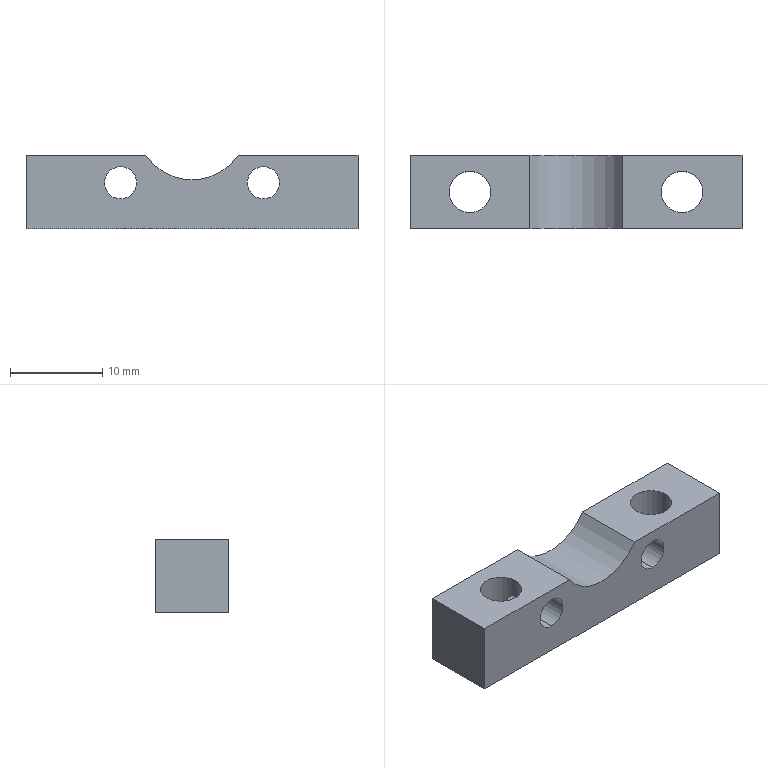Part | 1 solid | 22 faces | box 36 x 8 x 8 mm | volume 1705 mm3 | cylinder 13 | plane 9 | commonest cylinder face diameters 3.5 x4 4.5 x4 5 x4 12 x1
STEP:
#1=CARTESIAN_POINT('',(-7.75,2.,2.5));
#2=VERTEX_POINT('',#1);
#3=CARTESIAN_POINT('',(-7.75,2.,7.5));
#4=VERTEX_POINT('',#3);
#5=CARTESIAN_POINT('',(-7.75,2.,5.));
#6=DIRECTION('',(0.,1.,0.));
#7=DIRECTION('',(0.,0.,1.));
#8=AXIS2_PLACEMENT_3D('',#5,#6,#7);
#9=CIRCLE('',#8,2.5);
#10=EDGE_CURVE('',#2,#4,#9,.T.);
#11=ORIENTED_EDGE('',*,*,#10,.F.);
#12=CARTESIAN_POINT('',(-7.75,4.,2.5));
#13=VERTEX_POINT('',#12);
#14=CARTESIAN_POINT('',(-7.75,4.,2.5));
#15=DIRECTION('',(0.,1.,0.));
#16=VECTOR('',#15,1000.);
#17=LINE('',#14,#16);
#18=EDGE_CURVE('',#2,#13,#17,.T.);
#19=ORIENTED_EDGE('',*,*,#18,.T.);
#20=CARTESIAN_POINT('',(-7.75,4.,7.5));
#21=VERTEX_POINT('',#20);
#22=CARTESIAN_POINT('',(-7.75,4.,5.));
#23=DIRECTION('',(0.,1.,0.));
#24=DIRECTION('',(0.,0.,1.));
#25=AXIS2_PLACEMENT_3D('',#22,#23,#24);
#26=CIRCLE('',#25,2.5);
#27=EDGE_CURVE('',#13,#21,#26,.T.);
#28=ORIENTED_EDGE('',*,*,#27,.T.);
#29=CARTESIAN_POINT('',(-7.75,4.,7.5));
#30=DIRECTION('',(0.,1.,0.));
#31=VECTOR('',#30,1000.);
#32=LINE('',#29,#31);
#33=EDGE_CURVE('',#4,#21,#32,.T.);
#34=ORIENTED_EDGE('',*,*,#33,.F.);
#35=EDGE_LOOP('',(#11,#19,#28,#34));
#36=FACE_OUTER_BOUND('',#35,.T.);
#37=CARTESIAN_POINT('',(-7.75,4.,5.));
#38=DIRECTION('',(0.,1.,0.));
#39=DIRECTION('',(0.,0.,1.));
#40=AXIS2_PLACEMENT_3D('',#37,#38,#39);
#41=CYLINDRICAL_SURFACE('',#40,2.5);
#42=ADVANCED_FACE('',(#36),#41,.F.);
#43=CARTESIAN_POINT('',(-9.25,0.,4.099));
#44=VERTEX_POINT('',#43);
#45=CARTESIAN_POINT('',(-9.25,0.,5.901));
#46=VERTEX_POINT('',#45);
#47=CARTESIAN_POINT('',(-9.25,0.,4.099));
#48=CARTESIAN_POINT('',(-9.25,0.1307,4.099));
#49=CARTESIAN_POINT('',(-9.262,0.2592,4.117));
#50=CARTESIAN_POINT('',(-9.304,0.5043,4.194));
#51=CARTESIAN_POINT('',(-9.334,0.6184,4.252));
#52=CARTESIAN_POINT('',(-9.383,0.7644,4.37));
#53=CARTESIAN_POINT('',(-9.4,0.8082,4.414));
#54=CARTESIAN_POINT('',(-9.431,0.8861,4.512));
#55=CARTESIAN_POINT('',(-9.447,0.9202,4.567));
#56=CARTESIAN_POINT('',(-9.484,1.002,4.738));
#57=CARTESIAN_POINT('',(-9.5,1.03,4.868));
#58=CARTESIAN_POINT('',(-9.5,1.031,5.127));
#59=CARTESIAN_POINT('',(-9.485,1.003,5.257));
#60=CARTESIAN_POINT('',(-9.434,0.8941,5.489));
#61=CARTESIAN_POINT('',(-9.4,0.8139,5.59));
#62=CARTESIAN_POINT('',(-9.334,0.6194,5.748));
#63=CARTESIAN_POINT('',(-9.304,0.5043,5.806));
#64=CARTESIAN_POINT('',(-9.262,0.2597,5.883));
#65=CARTESIAN_POINT('',(-9.25,0.1302,5.901));
#66=CARTESIAN_POINT('',(-9.25,0.,5.901));
#67=B_SPLINE_CURVE_WITH_KNOTS('',3,(#47,#48,#49,#50,#51,#52,#53,#54,#55,#56,#57,#58,#59,#60,#61,#62,#63,#64,#65,#66),.UNSPECIFIED.,.F.,.F.,(4,2,2,2,2,2,2,2,2,4),(0.,0.0003875,0.000775,0.0009687,0.001162,0.00155,0.001937,0.002325,0.002712,0.0031),.UNSPECIFIED.);
#68=EDGE_CURVE('',#44,#46,#67,.T.);
#69=ORIENTED_EDGE('',*,*,#68,.F.);
#70=CARTESIAN_POINT('',(-9.25,0.,5.901));
#71=CARTESIAN_POINT('',(-9.25,-0.13,5.901));
#72=CARTESIAN_POINT('',(-9.261,-0.2584,5.883));
#73=CARTESIAN_POINT('',(-9.304,-0.5033,5.807));
#74=CARTESIAN_POINT('',(-9.334,-0.6163,5.75));
#75=CARTESIAN_POINT('',(-9.399,-0.8123,5.592));
#76=CARTESIAN_POINT('',(-9.433,-0.8916,5.493));
#77=CARTESIAN_POINT('',(-9.472,-0.9743,5.319));
#78=CARTESIAN_POINT('',(-9.482,-0.995,5.259));
#79=CARTESIAN_POINT('',(-9.496,-1.023,5.134));
#80=CARTESIAN_POINT('',(-9.5,-1.031,5.068));
#81=CARTESIAN_POINT('',(-9.5,-1.031,4.874));
#82=CARTESIAN_POINT('',(-9.485,-1.003,4.744));
#83=CARTESIAN_POINT('',(-9.435,-0.8952,4.513));
#84=CARTESIAN_POINT('',(-9.4,-0.815,4.411));
#85=CARTESIAN_POINT('',(-9.335,-0.6199,4.252));
#86=CARTESIAN_POINT('',(-9.304,-0.5049,4.194));
#87=CARTESIAN_POINT('',(-9.262,-0.2612,4.117));
#88=CARTESIAN_POINT('',(-9.25,-0.1305,4.099));
#89=CARTESIAN_POINT('',(-9.25,0.,4.099));
#90=B_SPLINE_CURVE_WITH_KNOTS('',3,(#70,#71,#72,#73,#74,#75,#76,#77,#78,#79,#80,#81,#82,#83,#84,#85,#86,#87,#88,#89),.UNSPECIFIED.,.F.,.F.,(4,2,2,2,2,2,2,2,2,4),(0.0031,0.003487,0.003874,0.004261,0.004454,0.004647,0.005034,0.005421,0.005808,0.006195),.UNSPECIFIED.);
#91=EDGE_CURVE('',#46,#44,#90,.T.);
#92=ORIENTED_EDGE('',*,*,#91,.F.);
#93=EDGE_LOOP('',(#69,#92));
#94=FACE_BOUND('',#93,.T.);
#95=CARTESIAN_POINT('',(-7.75,-4.,3.25));
#96=VERTEX_POINT('',#95);
#97=CARTESIAN_POINT('',(-7.75,-4.,6.75));
#98=VERTEX_POINT('',#97);
#99=CARTESIAN_POINT('',(-7.75,-4.,5.));
#100=DIRECTION('',(0.,1.,0.));
#101=DIRECTION('',(0.,0.,1.));
#102=AXIS2_PLACEMENT_3D('',#99,#100,#101);
#103=CIRCLE('',#102,1.75);
#104=EDGE_CURVE('',#96,#98,#103,.T.);
#105=ORIENTED_EDGE('',*,*,#104,.F.);
#106=CARTESIAN_POINT('',(-7.75,2.,3.25));
#107=VERTEX_POINT('',#106);
#108=CARTESIAN_POINT('',(-7.75,4.,3.25));
#109=DIRECTION('',(0.,1.,0.));
#110=VECTOR('',#109,1000.);
#111=LINE('',#108,#110);
#112=EDGE_CURVE('',#96,#107,#111,.T.);
#113=ORIENTED_EDGE('',*,*,#112,.T.);
#114=CARTESIAN_POINT('',(-7.75,2.,6.75));
#115=VERTEX_POINT('',#114);
#116=CARTESIAN_POINT('',(-7.75,2.,5.));
#117=DIRECTION('',(0.,1.,0.));
#118=DIRECTION('',(0.,0.,1.));
#119=AXIS2_PLACEMENT_3D('',#116,#117,#118);
#120=CIRCLE('',#119,1.75);
#121=EDGE_CURVE('',#107,#115,#120,.T.);
#122=ORIENTED_EDGE('',*,*,#121,.T.);
#123=CARTESIAN_POINT('',(-7.75,4.,6.75));
#124=DIRECTION('',(0.,1.,0.));
#125=VECTOR('',#124,1000.);
#126=LINE('',#123,#125);
#127=EDGE_CURVE('',#98,#115,#126,.T.);
#128=ORIENTED_EDGE('',*,*,#127,.F.);
#129=EDGE_LOOP('',(#105,#113,#122,#128));
#130=FACE_OUTER_BOUND('',#129,.T.);
#131=CARTESIAN_POINT('',(-7.75,4.,5.));
#132=DIRECTION('',(0.,1.,0.));
#133=DIRECTION('',(0.,0.,1.));
#134=AXIS2_PLACEMENT_3D('',#131,#132,#133);
#135=CYLINDRICAL_SURFACE('',#134,1.75);
#136=ADVANCED_FACE('',(#94,#130),#135,.F.);
#137=CARTESIAN_POINT('',(7.75,2.,2.5));
#138=VERTEX_POINT('',#137);
#139=CARTESIAN_POINT('',(7.75,2.,7.5));
#140=VERTEX_POINT('',#139);
#141=CARTESIAN_POINT('',(7.75,2.,5.));
#142=DIRECTION('',(0.,1.,0.));
#143=DIRECTION('',(0.,0.,1.));
#144=AXIS2_PLACEMENT_3D('',#141,#142,#143);
#145=CIRCLE('',#144,2.5);
#146=EDGE_CURVE('',#138,#140,#145,.T.);
#147=ORIENTED_EDGE('',*,*,#146,.F.);
#148=CARTESIAN_POINT('',(7.75,4.,2.5));
#149=VERTEX_POINT('',#148);
#150=CARTESIAN_POINT('',(7.75,4.,2.5));
#151=DIRECTION('',(0.,1.,0.));
#152=VECTOR('',#151,1000.);
#153=LINE('',#150,#152);
#154=EDGE_CURVE('',#138,#149,#153,.T.);
#155=ORIENTED_EDGE('',*,*,#154,.T.);
#156=CARTESIAN_POINT('',(7.75,4.,7.5));
#157=VERTEX_POINT('',#156);
#158=CARTESIAN_POINT('',(7.75,4.,5.));
#159=DIRECTION('',(0.,1.,0.));
#160=DIRECTION('',(0.,0.,1.));
#161=AXIS2_PLACEMENT_3D('',#158,#159,#160);
#162=CIRCLE('',#161,2.5);
#163=EDGE_CURVE('',#149,#157,#162,.T.);
#164=ORIENTED_EDGE('',*,*,#163,.T.);
#165=CARTESIAN_POINT('',(7.75,4.,7.5));
#166=DIRECTION('',(0.,1.,0.));
#167=VECTOR('',#166,1000.);
#168=LINE('',#165,#167);
#169=EDGE_CURVE('',#140,#157,#168,.T.);
#170=ORIENTED_EDGE('',*,*,#169,.F.);
#171=EDGE_LOOP('',(#147,#155,#164,#170));
#172=FACE_OUTER_BOUND('',#171,.T.);
#173=CARTESIAN_POINT('',(7.75,4.,5.));
#174=DIRECTION('',(0.,1.,0.));
#175=DIRECTION('',(0.,0.,1.));
#176=AXIS2_PLACEMENT_3D('',#173,#174,#175);
#177=CYLINDRICAL_SURFACE('',#176,2.5);
#178=ADVANCED_FACE('',(#172),#177,.F.);
#179=CARTESIAN_POINT('',(7.75,-4.,3.25));
#180=VERTEX_POINT('',#179);
#181=CARTESIAN_POINT('',(7.75,-4.,6.75));
#182=VERTEX_POINT('',#181);
#183=CARTESIAN_POINT('',(7.75,-4.,5.));
#184=DIRECTION('',(0.,1.,0.));
#185=DIRECTION('',(0.,0.,1.));
#186=AXIS2_PLACEMENT_3D('',#183,#184,#185);
#187=CIRCLE('',#186,1.75);
#188=EDGE_CURVE('',#180,#182,#187,.T.);
#189=ORIENTED_EDGE('',*,*,#188,.F.);
#190=CARTESIAN_POINT('',(7.75,2.,3.25));
#191=VERTEX_POINT('',#190);
#192=CARTESIAN_POINT('',(7.75,4.,3.25));
#193=DIRECTION('',(0.,1.,0.));
#194=VECTOR('',#193,1000.);
#195=LINE('',#192,#194);
#196=EDGE_CURVE('',#180,#191,#195,.T.);
#197=ORIENTED_EDGE('',*,*,#196,.T.);
#198=CARTESIAN_POINT('',(7.75,2.,6.75));
#199=VERTEX_POINT('',#198);
#200=CARTESIAN_POINT('',(7.75,2.,5.));
#201=DIRECTION('',(0.,1.,0.));
#202=DIRECTION('',(0.,0.,1.));
#203=AXIS2_PLACEMENT_3D('',#200,#201,#202);
#204=CIRCLE('',#203,1.75);
#205=EDGE_CURVE('',#191,#199,#204,.T.);
#206=ORIENTED_EDGE('',*,*,#205,.T.);
#207=CARTESIAN_POINT('',(7.75,4.,6.75));
#208=DIRECTION('',(0.,1.,0.));
#209=VECTOR('',#208,1000.);
#210=LINE('',#207,#209);
#211=EDGE_CURVE('',#182,#199,#210,.T.);
#212=ORIENTED_EDGE('',*,*,#211,.F.);
#213=EDGE_LOOP('',(#189,#197,#206,#212));
#214=FACE_OUTER_BOUND('',#213,.T.);
#215=CARTESIAN_POINT('',(7.75,4.,5.));
#216=DIRECTION('',(0.,1.,0.));
#217=DIRECTION('',(0.,0.,1.));
#218=AXIS2_PLACEMENT_3D('',#215,#216,#217);
#219=CYLINDRICAL_SURFACE('',#218,1.75);
#220=ADVANCED_FACE('',(#214),#219,.F.);
#221=CARTESIAN_POINT('',(-13.75,0.,0.));
#222=VERTEX_POINT('',#221);
#223=CARTESIAN_POINT('',(-9.25,0.,0.));
#224=VERTEX_POINT('',#223);
#225=CARTESIAN_POINT('',(-11.5,0.,0.));
#226=DIRECTION('',(0.,0.,1.));
#227=DIRECTION('',(1.,0.,0.));
#228=AXIS2_PLACEMENT_3D('',#225,#226,#227);
#229=CIRCLE('',#228,2.25);
#230=EDGE_CURVE('',#222,#224,#229,.T.);
#231=ORIENTED_EDGE('',*,*,#230,.F.);
#232=CARTESIAN_POINT('',(-13.75,0.,8.));
#233=VERTEX_POINT('',#232);
#234=CARTESIAN_POINT('',(-13.75,0.,8.));
#235=DIRECTION('',(0.,0.,1.));
#236=VECTOR('',#235,1000.);
#237=LINE('',#234,#236);
#238=EDGE_CURVE('',#222,#233,#237,.T.);
#239=ORIENTED_EDGE('',*,*,#238,.T.);
#240=CARTESIAN_POINT('',(-9.25,0.,8.));
#241=VERTEX_POINT('',#240);
#242=CARTESIAN_POINT('',(-11.5,0.,8.));
#243=DIRECTION('',(0.,0.,1.));
#244=DIRECTION('',(1.,0.,0.));
#245=AXIS2_PLACEMENT_3D('',#242,#243,#244);
#246=CIRCLE('',#245,2.25);
#247=EDGE_CURVE('',#233,#241,#246,.T.);
#248=ORIENTED_EDGE('',*,*,#247,.T.);
#249=CARTESIAN_POINT('',(-9.25,0.,8.));
#250=DIRECTION('',(0.,0.,1.));
#251=VECTOR('',#250,1000.);
#252=LINE('',#249,#251);
#253=EDGE_CURVE('',#46,#241,#252,.T.);
#254=ORIENTED_EDGE('',*,*,#253,.F.);
#255=ORIENTED_EDGE('',*,*,#91,.T.);
#256=CARTESIAN_POINT('',(-9.25,0.,8.));
#257=DIRECTION('',(0.,0.,1.));
#258=VECTOR('',#257,1000.);
#259=LINE('',#256,#258);
#260=EDGE_CURVE('',#224,#44,#259,.T.);
#261=ORIENTED_EDGE('',*,*,#260,.F.);
#262=EDGE_LOOP('',(#231,#239,#248,#254,#255,#261));
#263=FACE_OUTER_BOUND('',#262,.T.);
#264=CARTESIAN_POINT('',(-11.5,0.,8.));
#265=DIRECTION('',(0.,0.,1.));
#266=DIRECTION('',(1.,0.,0.));
#267=AXIS2_PLACEMENT_3D('',#264,#265,#266);
#268=CYLINDRICAL_SURFACE('',#267,2.25);
#269=ADVANCED_FACE('',(#263),#268,.F.);
#270=CARTESIAN_POINT('',(13.75,0.,8.));
#271=VERTEX_POINT('',#270);
#272=CARTESIAN_POINT('',(9.25,0.,8.));
#273=VERTEX_POINT('',#272);
#274=CARTESIAN_POINT('',(11.5,0.,8.));
#275=DIRECTION('',(0.,0.,-1.));
#276=DIRECTION('',(-1.,0.,0.));
#277=AXIS2_PLACEMENT_3D('',#274,#275,#276);
#278=CIRCLE('',#277,2.25);
#279=EDGE_CURVE('',#271,#273,#278,.T.);
#280=ORIENTED_EDGE('',*,*,#279,.F.);
#281=CARTESIAN_POINT('',(13.75,0.,0.));
#282=VERTEX_POINT('',#281);
#283=CARTESIAN_POINT('',(13.75,0.,0.));
#284=DIRECTION('',(0.,0.,-1.));
#285=VECTOR('',#284,1000.);
#286=LINE('',#283,#285);
#287=EDGE_CURVE('',#271,#282,#286,.T.);
#288=ORIENTED_EDGE('',*,*,#287,.T.);
#289=CARTESIAN_POINT('',(9.25,0.,0.));
#290=VERTEX_POINT('',#289);
#291=CARTESIAN_POINT('',(11.5,0.,0.));
#292=DIRECTION('',(0.,0.,-1.));
#293=DIRECTION('',(-1.,0.,0.));
#294=AXIS2_PLACEMENT_3D('',#291,#292,#293);
#295=CIRCLE('',#294,2.25);
#296=EDGE_CURVE('',#282,#290,#295,.T.);
#297=ORIENTED_EDGE('',*,*,#296,.T.);
#298=CARTESIAN_POINT('',(9.25,0.,4.099));
#299=VERTEX_POINT('',#298);
#300=CARTESIAN_POINT('',(9.25,0.,0.));
#301=DIRECTION('',(0.,0.,-1.));
#302=VECTOR('',#301,1000.);
#303=LINE('',#300,#302);
#304=EDGE_CURVE('',#299,#290,#303,.T.);
#305=ORIENTED_EDGE('',*,*,#304,.F.);
#306=CARTESIAN_POINT('',(9.25,0.,5.901));
#307=VERTEX_POINT('',#306);
#308=CARTESIAN_POINT('',(9.25,0.,4.099));
#309=CARTESIAN_POINT('',(9.25,-0.13,4.099));
#310=CARTESIAN_POINT('',(9.261,-0.2584,4.117));
#311=CARTESIAN_POINT('',(9.304,-0.5033,4.193));
#312=CARTESIAN_POINT('',(9.334,-0.6163,4.25));
#313=CARTESIAN_POINT('',(9.399,-0.8123,4.408));
#314=CARTESIAN_POINT('',(9.433,-0.8916,4.507));
#315=CARTESIAN_POINT('',(9.472,-0.9743,4.681));
#316=CARTESIAN_POINT('',(9.482,-0.995,4.741));
#317=CARTESIAN_POINT('',(9.496,-1.023,4.866));
#318=CARTESIAN_POINT('',(9.5,-1.031,4.932));
#319=CARTESIAN_POINT('',(9.5,-1.031,5.126));
#320=CARTESIAN_POINT('',(9.485,-1.003,5.256));
#321=CARTESIAN_POINT('',(9.435,-0.8952,5.487));
#322=CARTESIAN_POINT('',(9.4,-0.815,5.589));
#323=CARTESIAN_POINT('',(9.335,-0.6199,5.748));
#324=CARTESIAN_POINT('',(9.304,-0.5049,5.806));
#325=CARTESIAN_POINT('',(9.262,-0.2612,5.883));
#326=CARTESIAN_POINT('',(9.25,-0.1305,5.901));
#327=CARTESIAN_POINT('',(9.25,0.,5.901));
#328=B_SPLINE_CURVE_WITH_KNOTS('',3,(#308,#309,#310,#311,#312,#313,#314,#315,#316,#317,#318,#319,#320,#321,#322,#323,#324,#325,#326,#327),.UNSPECIFIED.,.F.,.F.,(4,2,2,2,2,2,2,2,2,4),(0.0031,0.003487,0.003874,0.004261,0.004454,0.004647,0.005034,0.005421,0.005808,0.006195),.UNSPECIFIED.);
#329=EDGE_CURVE('',#299,#307,#328,.T.);
#330=ORIENTED_EDGE('',*,*,#329,.T.);
#331=CARTESIAN_POINT('',(9.25,0.,0.));
#332=DIRECTION('',(0.,0.,-1.));
#333=VECTOR('',#332,1000.);
#334=LINE('',#331,#333);
#335=EDGE_CURVE('',#273,#307,#334,.T.);
#336=ORIENTED_EDGE('',*,*,#335,.F.);
#337=EDGE_LOOP('',(#280,#288,#297,#305,#330,#336));
#338=FACE_OUTER_BOUND('',#337,.T.);
#339=CARTESIAN_POINT('',(11.5,0.,0.));
#340=DIRECTION('',(0.,0.,-1.));
#341=DIRECTION('',(-1.,0.,0.));
#342=AXIS2_PLACEMENT_3D('',#339,#340,#341);
#343=CYLINDRICAL_SURFACE('',#342,2.25);
#344=ADVANCED_FACE('',(#338),#343,.F.);
#345=CARTESIAN_POINT('',(11.5,0.,8.));
#346=DIRECTION('',(0.,0.,-1.));
#347=DIRECTION('',(-1.,0.,0.));
#348=AXIS2_PLACEMENT_3D('',#345,#346,#347);
#349=CIRCLE('',#348,2.25);
#350=EDGE_CURVE('',#273,#271,#349,.T.);
#351=ORIENTED_EDGE('',*,*,#350,.T.);
#352=ORIENTED_EDGE('',*,*,#279,.T.);
#353=EDGE_LOOP('',(#351,#352));
#354=FACE_BOUND('',#353,.T.);
#355=CARTESIAN_POINT('',(5.,-4.,8.));
#356=VERTEX_POINT('',#355);
#357=CARTESIAN_POINT('',(5.,4.,8.));
#358=VERTEX_POINT('',#357);
#359=CARTESIAN_POINT('',(5.,-4.,8.));
#360=DIRECTION('',(0.,1.,0.));
#361=VECTOR('',#360,1000.);
#362=LINE('',#359,#361);
#363=EDGE_CURVE('',#356,#358,#362,.T.);
#364=ORIENTED_EDGE('',*,*,#363,.F.);
#365=CARTESIAN_POINT('',(18.,-4.,8.));
#366=VERTEX_POINT('',#365);
#367=CARTESIAN_POINT('',(18.,-4.,8.));
#368=DIRECTION('',(-1.,0.,0.));
#369=VECTOR('',#368,1000.);
#370=LINE('',#367,#369);
#371=EDGE_CURVE('',#366,#356,#370,.T.);
#372=ORIENTED_EDGE('',*,*,#371,.F.);
#373=CARTESIAN_POINT('',(18.,4.,8.));
#374=VERTEX_POINT('',#373);
#375=CARTESIAN_POINT('',(18.,4.,8.));
#376=DIRECTION('',(0.,-1.,0.));
#377=VECTOR('',#376,1000.);
#378=LINE('',#375,#377);
#379=EDGE_CURVE('',#374,#366,#378,.T.);
#380=ORIENTED_EDGE('',*,*,#379,.F.);
#381=CARTESIAN_POINT('',(18.,4.,8.));
#382=DIRECTION('',(-1.,0.,0.));
#383=VECTOR('',#382,1000.);
#384=LINE('',#381,#383);
#385=EDGE_CURVE('',#374,#358,#384,.T.);
#386=ORIENTED_EDGE('',*,*,#385,.T.);
#387=EDGE_LOOP('',(#364,#372,#380,#386));
#388=FACE_OUTER_BOUND('',#387,.T.);
#389=CARTESIAN_POINT('',(18.,4.,8.));
#390=DIRECTION('',(0.,0.,1.));
#391=DIRECTION('',(1.,0.,0.));
#392=AXIS2_PLACEMENT_3D('',#389,#390,#391);
#393=PLANE('',#392);
#394=ADVANCED_FACE('',(#354,#388),#393,.T.);
#395=CARTESIAN_POINT('',(-11.5,0.,0.));
#396=DIRECTION('',(0.,0.,1.));
#397=DIRECTION('',(1.,0.,0.));
#398=AXIS2_PLACEMENT_3D('',#395,#396,#397);
#399=CIRCLE('',#398,2.25);
#400=EDGE_CURVE('',#224,#222,#399,.T.);
#401=ORIENTED_EDGE('',*,*,#400,.T.);
#402=ORIENTED_EDGE('',*,*,#230,.T.);
#403=EDGE_LOOP('',(#401,#402));
#404=FACE_BOUND('',#403,.T.);
#405=CARTESIAN_POINT('',(11.5,0.,0.));
#406=DIRECTION('',(0.,0.,-1.));
#407=DIRECTION('',(-1.,0.,0.));
#408=AXIS2_PLACEMENT_3D('',#405,#406,#407);
#409=CIRCLE('',#408,2.25);
#410=EDGE_CURVE('',#290,#282,#409,.T.);
#411=ORIENTED_EDGE('',*,*,#410,.F.);
#412=ORIENTED_EDGE('',*,*,#296,.F.);
#413=EDGE_LOOP('',(#411,#412));
#414=FACE_BOUND('',#413,.T.);
#415=CARTESIAN_POINT('',(-18.,-4.,0.));
#416=VERTEX_POINT('',#415);
#417=CARTESIAN_POINT('',(18.,-4.,0.));
#418=VERTEX_POINT('',#417);
#419=CARTESIAN_POINT('',(-18.,-4.,0.));
#420=DIRECTION('',(1.,0.,0.));
#421=VECTOR('',#420,1000.);
#422=LINE('',#419,#421);
#423=EDGE_CURVE('',#416,#418,#422,.T.);
#424=ORIENTED_EDGE('',*,*,#423,.F.);
#425=CARTESIAN_POINT('',(-18.,4.,0.));
#426=VERTEX_POINT('',#425);
#427=CARTESIAN_POINT('',(-18.,4.,0.));
#428=DIRECTION('',(0.,-1.,0.));
#429=VECTOR('',#428,1000.);
#430=LINE('',#427,#429);
#431=EDGE_CURVE('',#426,#416,#430,.T.);
#432=ORIENTED_EDGE('',*,*,#431,.F.);
#433=CARTESIAN_POINT('',(18.,4.,0.));
#434=VERTEX_POINT('',#433);
#435=CARTESIAN_POINT('',(-18.,4.,0.));
#436=DIRECTION('',(1.,0.,0.));
#437=VECTOR('',#436,1000.);
#438=LINE('',#435,#437);
#439=EDGE_CURVE('',#426,#434,#438,.T.);
#440=ORIENTED_EDGE('',*,*,#439,.T.);
#441=CARTESIAN_POINT('',(18.,4.,0.));
#442=DIRECTION('',(0.,-1.,0.));
#443=VECTOR('',#442,1000.);
#444=LINE('',#441,#443);
#445=EDGE_CURVE('',#434,#418,#444,.T.);
#446=ORIENTED_EDGE('',*,*,#445,.T.);
#447=EDGE_LOOP('',(#424,#432,#440,#446));
#448=FACE_OUTER_BOUND('',#447,.T.);
#449=CARTESIAN_POINT('',(-18.,4.,0.));
#450=DIRECTION('',(0.,0.,-1.));
#451=DIRECTION('',(-1.,0.,0.));
#452=AXIS2_PLACEMENT_3D('',#449,#450,#451);
#453=PLANE('',#452);
#454=ADVANCED_FACE('',(#404,#414,#448),#453,.T.);
#455=CARTESIAN_POINT('',(-18.,-4.,8.));
#456=VERTEX_POINT('',#455);
#457=CARTESIAN_POINT('',(-18.,-4.,8.));
#458=DIRECTION('',(0.,0.,-1.));
#459=VECTOR('',#458,1000.);
#460=LINE('',#457,#459);
#461=EDGE_CURVE('',#456,#416,#460,.T.);
#462=ORIENTED_EDGE('',*,*,#461,.F.);
#463=CARTESIAN_POINT('',(-18.,4.,8.));
#464=VERTEX_POINT('',#463);
#465=CARTESIAN_POINT('',(-18.,4.,8.));
#466=DIRECTION('',(0.,-1.,0.));
#467=VECTOR('',#466,1000.);
#468=LINE('',#465,#467);
#469=EDGE_CURVE('',#464,#456,#468,.T.);
#470=ORIENTED_EDGE('',*,*,#469,.F.);
#471=CARTESIAN_POINT('',(-18.,4.,8.));
#472=DIRECTION('',(0.,0.,-1.));
#473=VECTOR('',#472,1000.);
#474=LINE('',#471,#473);
#475=EDGE_CURVE('',#464,#426,#474,.T.);
#476=ORIENTED_EDGE('',*,*,#475,.T.);
#477=ORIENTED_EDGE('',*,*,#431,.T.);
#478=EDGE_LOOP('',(#462,#470,#476,#477));
#479=FACE_OUTER_BOUND('',#478,.T.);
#480=CARTESIAN_POINT('',(-18.,4.,8.));
#481=DIRECTION('',(-1.,0.,0.));
#482=DIRECTION('',(0.,0.,1.));
#483=AXIS2_PLACEMENT_3D('',#480,#481,#482);
#484=PLANE('',#483);
#485=ADVANCED_FACE('',(#479),#484,.T.);
#486=CARTESIAN_POINT('',(-11.5,0.,8.));
#487=DIRECTION('',(0.,0.,1.));
#488=DIRECTION('',(1.,0.,0.));
#489=AXIS2_PLACEMENT_3D('',#486,#487,#488);
#490=CIRCLE('',#489,2.25);
#491=EDGE_CURVE('',#241,#233,#490,.T.);
#492=ORIENTED_EDGE('',*,*,#491,.F.);
#493=ORIENTED_EDGE('',*,*,#247,.F.);
#494=EDGE_LOOP('',(#492,#493));
#495=FACE_BOUND('',#494,.T.);
#496=CARTESIAN_POINT('',(-5.,-4.,8.));
#497=VERTEX_POINT('',#496);
#498=CARTESIAN_POINT('',(-5.,4.,8.));
#499=VERTEX_POINT('',#498);
#500=CARTESIAN_POINT('',(-5.,-4.,8.));
#501=DIRECTION('',(0.,1.,0.));
#502=VECTOR('',#501,1000.);
#503=LINE('',#500,#502);
#504=EDGE_CURVE('',#497,#499,#503,.T.);
#505=ORIENTED_EDGE('',*,*,#504,.T.);
#506=CARTESIAN_POINT('',(18.,4.,8.));
#507=DIRECTION('',(-1.,0.,0.));
#508=VECTOR('',#507,1000.);
#509=LINE('',#506,#508);
#510=EDGE_CURVE('',#499,#464,#509,.T.);
#511=ORIENTED_EDGE('',*,*,#510,.T.);
#512=ORIENTED_EDGE('',*,*,#469,.T.);
#513=CARTESIAN_POINT('',(18.,-4.,8.));
#514=DIRECTION('',(-1.,0.,0.));
#515=VECTOR('',#514,1000.);
#516=LINE('',#513,#515);
#517=EDGE_CURVE('',#497,#456,#516,.T.);
#518=ORIENTED_EDGE('',*,*,#517,.F.);
#519=EDGE_LOOP('',(#505,#511,#512,#518));
#520=FACE_OUTER_BOUND('',#519,.T.);
#521=CARTESIAN_POINT('',(18.,4.,8.));
#522=DIRECTION('',(0.,0.,1.));
#523=DIRECTION('',(1.,0.,0.));
#524=AXIS2_PLACEMENT_3D('',#521,#522,#523);
#525=PLANE('',#524);
#526=ADVANCED_FACE('',(#495,#520),#525,.T.);
#527=CARTESIAN_POINT('',(18.,-4.,0.));
#528=DIRECTION('',(0.,0.,1.));
#529=VECTOR('',#528,1000.);
#530=LINE('',#527,#529);
#531=EDGE_CURVE('',#418,#366,#530,.T.);
#532=ORIENTED_EDGE('',*,*,#531,.F.);
#533=ORIENTED_EDGE('',*,*,#445,.F.);
#534=CARTESIAN_POINT('',(18.,4.,0.));
#535=DIRECTION('',(0.,0.,1.));
#536=VECTOR('',#535,1000.);
#537=LINE('',#534,#536);
#538=EDGE_CURVE('',#434,#374,#537,.T.);
#539=ORIENTED_EDGE('',*,*,#538,.T.);
#540=ORIENTED_EDGE('',*,*,#379,.T.);
#541=EDGE_LOOP('',(#532,#533,#539,#540));
#542=FACE_OUTER_BOUND('',#541,.T.);
#543=CARTESIAN_POINT('',(18.,4.,0.));
#544=DIRECTION('',(1.,0.,0.));
#545=DIRECTION('',(0.,0.,-1.));
#546=AXIS2_PLACEMENT_3D('',#543,#544,#545);
#547=PLANE('',#546);
#548=ADVANCED_FACE('',(#542),#547,.T.);
#549=CARTESIAN_POINT('',(-7.75,4.,5.));
#550=DIRECTION('',(0.,1.,0.));
#551=DIRECTION('',(0.,0.,1.));
#552=AXIS2_PLACEMENT_3D('',#549,#550,#551);
#553=CIRCLE('',#552,2.5);
#554=EDGE_CURVE('',#21,#13,#553,.T.);
#555=ORIENTED_EDGE('',*,*,#554,.F.);
#556=ORIENTED_EDGE('',*,*,#27,.F.);
#557=EDGE_LOOP('',(#555,#556));
#558=FACE_BOUND('',#557,.T.);
#559=CARTESIAN_POINT('',(7.75,4.,5.));
#560=DIRECTION('',(0.,1.,0.));
#561=DIRECTION('',(0.,0.,1.));
#562=AXIS2_PLACEMENT_3D('',#559,#560,#561);
#563=CIRCLE('',#562,2.5);
#564=EDGE_CURVE('',#157,#149,#563,.T.);
#565=ORIENTED_EDGE('',*,*,#564,.F.);
#566=ORIENTED_EDGE('',*,*,#163,.F.);
#567=EDGE_LOOP('',(#565,#566));
#568=FACE_BOUND('',#567,.T.);
#569=ORIENTED_EDGE('',*,*,#510,.F.);
#570=CARTESIAN_POINT('',(0.,4.,11.317));
#571=DIRECTION('',(0.,1.,0.));
#572=DIRECTION('',(0.,0.,1.));
#573=AXIS2_PLACEMENT_3D('',#570,#571,#572);
#574=CIRCLE('',#573,6.);
#575=EDGE_CURVE('',#358,#499,#574,.T.);
#576=ORIENTED_EDGE('',*,*,#575,.F.);
#577=ORIENTED_EDGE('',*,*,#385,.F.);
#578=ORIENTED_EDGE('',*,*,#538,.F.);
#579=ORIENTED_EDGE('',*,*,#439,.F.);
#580=ORIENTED_EDGE('',*,*,#475,.F.);
#581=EDGE_LOOP('',(#569,#576,#577,#578,#579,#580));
#582=FACE_OUTER_BOUND('',#581,.T.);
#583=CARTESIAN_POINT('',(0.,4.,0.));
#584=DIRECTION('',(0.,-1.,0.));
#585=DIRECTION('',(0.,0.,-1.));
#586=AXIS2_PLACEMENT_3D('',#583,#584,#585);
#587=PLANE('',#586);
#588=ADVANCED_FACE('',(#558,#568,#582),#587,.F.);
#589=CARTESIAN_POINT('',(-7.75,-4.,5.));
#590=DIRECTION('',(0.,1.,0.));
#591=DIRECTION('',(0.,0.,1.));
#592=AXIS2_PLACEMENT_3D('',#589,#590,#591);
#593=CIRCLE('',#592,1.75);
#594=EDGE_CURVE('',#98,#96,#593,.T.);
#595=ORIENTED_EDGE('',*,*,#594,.T.);
#596=ORIENTED_EDGE('',*,*,#104,.T.);
#597=EDGE_LOOP('',(#595,#596));
#598=FACE_BOUND('',#597,.T.);
#599=CARTESIAN_POINT('',(7.75,-4.,5.));
#600=DIRECTION('',(0.,1.,0.));
#601=DIRECTION('',(0.,0.,1.));
#602=AXIS2_PLACEMENT_3D('',#599,#600,#601);
#603=CIRCLE('',#602,1.75);
#604=EDGE_CURVE('',#182,#180,#603,.T.);
#605=ORIENTED_EDGE('',*,*,#604,.T.);
#606=ORIENTED_EDGE('',*,*,#188,.T.);
#607=EDGE_LOOP('',(#605,#606));
#608=FACE_BOUND('',#607,.T.);
#609=CARTESIAN_POINT('',(0.,-4.,11.317));
#610=DIRECTION('',(0.,1.,0.));
#611=DIRECTION('',(0.,0.,1.));
#612=AXIS2_PLACEMENT_3D('',#609,#610,#611);
#613=CIRCLE('',#612,6.);
#614=EDGE_CURVE('',#356,#497,#613,.T.);
#615=ORIENTED_EDGE('',*,*,#614,.T.);
#616=ORIENTED_EDGE('',*,*,#517,.T.);
#617=ORIENTED_EDGE('',*,*,#461,.T.);
#618=ORIENTED_EDGE('',*,*,#423,.T.);
#619=ORIENTED_EDGE('',*,*,#531,.T.);
#620=ORIENTED_EDGE('',*,*,#371,.T.);
#621=EDGE_LOOP('',(#615,#616,#617,#618,#619,#620));
#622=FACE_OUTER_BOUND('',#621,.T.);
#623=CARTESIAN_POINT('',(0.,-4.,0.));
#624=DIRECTION('',(0.,-1.,0.));
#625=DIRECTION('',(0.,0.,-1.));
#626=AXIS2_PLACEMENT_3D('',#623,#624,#625);
#627=PLANE('',#626);
#628=ADVANCED_FACE('',(#598,#608,#622),#627,.T.);
#629=ORIENTED_EDGE('',*,*,#575,.T.);
#630=ORIENTED_EDGE('',*,*,#504,.F.);
#631=ORIENTED_EDGE('',*,*,#614,.F.);
#632=ORIENTED_EDGE('',*,*,#363,.T.);
#633=EDGE_LOOP('',(#629,#630,#631,#632));
#634=FACE_OUTER_BOUND('',#633,.T.);
#635=CARTESIAN_POINT('',(0.,-4.,11.317));
#636=DIRECTION('',(0.,1.,0.));
#637=DIRECTION('',(0.,0.,1.));
#638=AXIS2_PLACEMENT_3D('',#635,#636,#637);
#639=CYLINDRICAL_SURFACE('',#638,6.);
#640=ADVANCED_FACE('',(#634),#639,.F.);
#641=ORIENTED_EDGE('',*,*,#287,.F.);
#642=ORIENTED_EDGE('',*,*,#350,.F.);
#643=ORIENTED_EDGE('',*,*,#335,.T.);
#644=CARTESIAN_POINT('',(9.25,0.,5.901));
#645=CARTESIAN_POINT('',(9.25,0.1307,5.901));
#646=CARTESIAN_POINT('',(9.262,0.2592,5.883));
#647=CARTESIAN_POINT('',(9.304,0.5043,5.806));
#648=CARTESIAN_POINT('',(9.334,0.6184,5.748));
#649=CARTESIAN_POINT('',(9.383,0.7644,5.63));
#650=CARTESIAN_POINT('',(9.4,0.8082,5.586));
#651=CARTESIAN_POINT('',(9.431,0.8861,5.488));
#652=CARTESIAN_POINT('',(9.447,0.9202,5.433));
#653=CARTESIAN_POINT('',(9.484,1.002,5.262));
#654=CARTESIAN_POINT('',(9.5,1.03,5.132));
#655=CARTESIAN_POINT('',(9.5,1.031,4.873));
#656=CARTESIAN_POINT('',(9.485,1.003,4.743));
#657=CARTESIAN_POINT('',(9.434,0.8941,4.511));
#658=CARTESIAN_POINT('',(9.4,0.8139,4.41));
#659=CARTESIAN_POINT('',(9.334,0.6194,4.252));
#660=CARTESIAN_POINT('',(9.304,0.5043,4.194));
#661=CARTESIAN_POINT('',(9.262,0.2597,4.117));
#662=CARTESIAN_POINT('',(9.25,0.1302,4.099));
#663=CARTESIAN_POINT('',(9.25,0.,4.099));
#664=B_SPLINE_CURVE_WITH_KNOTS('',3,(#644,#645,#646,#647,#648,#649,#650,#651,#652,#653,#654,#655,#656,#657,#658,#659,#660,#661,#662,#663),.UNSPECIFIED.,.F.,.F.,(4,2,2,2,2,2,2,2,2,4),(0.,0.0003875,0.000775,0.0009687,0.001162,0.00155,0.001937,0.002325,0.002712,0.0031),.UNSPECIFIED.);
#665=EDGE_CURVE('',#307,#299,#664,.T.);
#666=ORIENTED_EDGE('',*,*,#665,.T.);
#667=ORIENTED_EDGE('',*,*,#304,.T.);
#668=ORIENTED_EDGE('',*,*,#410,.T.);
#669=EDGE_LOOP('',(#641,#642,#643,#666,#667,#668));
#670=FACE_OUTER_BOUND('',#669,.T.);
#671=CARTESIAN_POINT('',(11.5,0.,0.));
#672=DIRECTION('',(0.,0.,-1.));
#673=DIRECTION('',(-1.,0.,0.));
#674=AXIS2_PLACEMENT_3D('',#671,#672,#673);
#675=CYLINDRICAL_SURFACE('',#674,2.25);
#676=ADVANCED_FACE('',(#670),#675,.F.);
#677=ORIENTED_EDGE('',*,*,#238,.F.);
#678=ORIENTED_EDGE('',*,*,#400,.F.);
#679=ORIENTED_EDGE('',*,*,#260,.T.);
#680=ORIENTED_EDGE('',*,*,#68,.T.);
#681=ORIENTED_EDGE('',*,*,#253,.T.);
#682=ORIENTED_EDGE('',*,*,#491,.T.);
#683=EDGE_LOOP('',(#677,#678,#679,#680,#681,#682));
#684=FACE_OUTER_BOUND('',#683,.T.);
#685=CARTESIAN_POINT('',(-11.5,0.,8.));
#686=DIRECTION('',(0.,0.,1.));
#687=DIRECTION('',(1.,0.,0.));
#688=AXIS2_PLACEMENT_3D('',#685,#686,#687);
#689=CYLINDRICAL_SURFACE('',#688,2.25);
#690=ADVANCED_FACE('',(#684),#689,.F.);
#691=ORIENTED_EDGE('',*,*,#196,.F.);
#692=ORIENTED_EDGE('',*,*,#604,.F.);
#693=ORIENTED_EDGE('',*,*,#211,.T.);
#694=CARTESIAN_POINT('',(7.75,2.,5.));
#695=DIRECTION('',(0.,1.,0.));
#696=DIRECTION('',(0.,0.,1.));
#697=AXIS2_PLACEMENT_3D('',#694,#695,#696);
#698=CIRCLE('',#697,1.75);
#699=EDGE_CURVE('',#199,#191,#698,.T.);
#700=ORIENTED_EDGE('',*,*,#699,.T.);
#701=EDGE_LOOP('',(#691,#692,#693,#700));
#702=FACE_OUTER_BOUND('',#701,.T.);
#703=ORIENTED_EDGE('',*,*,#665,.F.);
#704=ORIENTED_EDGE('',*,*,#329,.F.);
#705=EDGE_LOOP('',(#703,#704));
#706=FACE_BOUND('',#705,.T.);
#707=CARTESIAN_POINT('',(7.75,4.,5.));
#708=DIRECTION('',(0.,1.,0.));
#709=DIRECTION('',(0.,0.,1.));
#710=AXIS2_PLACEMENT_3D('',#707,#708,#709);
#711=CYLINDRICAL_SURFACE('',#710,1.75);
#712=ADVANCED_FACE('',(#702,#706),#711,.F.);
#713=ORIENTED_EDGE('',*,*,#699,.F.);
#714=ORIENTED_EDGE('',*,*,#205,.F.);
#715=EDGE_LOOP('',(#713,#714));
#716=FACE_BOUND('',#715,.T.);
#717=CARTESIAN_POINT('',(7.75,2.,5.));
#718=DIRECTION('',(0.,1.,0.));
#719=DIRECTION('',(0.,0.,1.));
#720=AXIS2_PLACEMENT_3D('',#717,#718,#719);
#721=CIRCLE('',#720,2.5);
#722=EDGE_CURVE('',#140,#138,#721,.T.);
#723=ORIENTED_EDGE('',*,*,#722,.T.);
#724=ORIENTED_EDGE('',*,*,#146,.T.);
#725=EDGE_LOOP('',(#723,#724));
#726=FACE_OUTER_BOUND('',#725,.T.);
#727=CARTESIAN_POINT('',(9.5,2.,5.));
#728=DIRECTION('',(0.,-1.,0.));
#729=DIRECTION('',(0.,0.,-1.));
#730=AXIS2_PLACEMENT_3D('',#727,#728,#729);
#731=PLANE('',#730);
#732=ADVANCED_FACE('',(#716,#726),#731,.F.);
#733=ORIENTED_EDGE('',*,*,#154,.F.);
#734=ORIENTED_EDGE('',*,*,#722,.F.);
#735=ORIENTED_EDGE('',*,*,#169,.T.);
#736=ORIENTED_EDGE('',*,*,#564,.T.);
#737=EDGE_LOOP('',(#733,#734,#735,#736));
#738=FACE_OUTER_BOUND('',#737,.T.);
#739=CARTESIAN_POINT('',(7.75,4.,5.));
#740=DIRECTION('',(0.,1.,0.));
#741=DIRECTION('',(0.,0.,1.));
#742=AXIS2_PLACEMENT_3D('',#739,#740,#741);
#743=CYLINDRICAL_SURFACE('',#742,2.5);
#744=ADVANCED_FACE('',(#738),#743,.F.);
#745=ORIENTED_EDGE('',*,*,#112,.F.);
#746=ORIENTED_EDGE('',*,*,#594,.F.);
#747=ORIENTED_EDGE('',*,*,#127,.T.);
#748=CARTESIAN_POINT('',(-7.75,2.,5.));
#749=DIRECTION('',(0.,1.,0.));
#750=DIRECTION('',(0.,0.,1.));
#751=AXIS2_PLACEMENT_3D('',#748,#749,#750);
#752=CIRCLE('',#751,1.75);
#753=EDGE_CURVE('',#115,#107,#752,.T.);
#754=ORIENTED_EDGE('',*,*,#753,.T.);
#755=EDGE_LOOP('',(#745,#746,#747,#754));
#756=FACE_OUTER_BOUND('',#755,.T.);
#757=CARTESIAN_POINT('',(-7.75,4.,5.));
#758=DIRECTION('',(0.,1.,0.));
#759=DIRECTION('',(0.,0.,1.));
#760=AXIS2_PLACEMENT_3D('',#757,#758,#759);
#761=CYLINDRICAL_SURFACE('',#760,1.75);
#762=ADVANCED_FACE('',(#756),#761,.F.);
#763=ORIENTED_EDGE('',*,*,#753,.F.);
#764=ORIENTED_EDGE('',*,*,#121,.F.);
#765=EDGE_LOOP('',(#763,#764));
#766=FACE_BOUND('',#765,.T.);
#767=CARTESIAN_POINT('',(-7.75,2.,5.));
#768=DIRECTION('',(0.,1.,0.));
#769=DIRECTION('',(0.,0.,1.));
#770=AXIS2_PLACEMENT_3D('',#767,#768,#769);
#771=CIRCLE('',#770,2.5);
#772=EDGE_CURVE('',#4,#2,#771,.T.);
#773=ORIENTED_EDGE('',*,*,#772,.T.);
#774=ORIENTED_EDGE('',*,*,#10,.T.);
#775=EDGE_LOOP('',(#773,#774));
#776=FACE_OUTER_BOUND('',#775,.T.);
#777=CARTESIAN_POINT('',(-6.,2.,5.));
#778=DIRECTION('',(0.,-1.,0.));
#779=DIRECTION('',(0.,0.,-1.));
#780=AXIS2_PLACEMENT_3D('',#777,#778,#779);
#781=PLANE('',#780);
#782=ADVANCED_FACE('',(#766,#776),#781,.F.);
#783=ORIENTED_EDGE('',*,*,#18,.F.);
#784=ORIENTED_EDGE('',*,*,#772,.F.);
#785=ORIENTED_EDGE('',*,*,#33,.T.);
#786=ORIENTED_EDGE('',*,*,#554,.T.);
#787=EDGE_LOOP('',(#783,#784,#785,#786));
#788=FACE_OUTER_BOUND('',#787,.T.);
#789=CARTESIAN_POINT('',(-7.75,4.,5.));
#790=DIRECTION('',(0.,1.,0.));
#791=DIRECTION('',(0.,0.,1.));
#792=AXIS2_PLACEMENT_3D('',#789,#790,#791);
#793=CYLINDRICAL_SURFACE('',#792,2.5);
#794=ADVANCED_FACE('',(#788),#793,.F.);
#795=CLOSED_SHELL('',(#42,#136,#178,#220,#269,#344,#394,#454,#485,#526,#548,#588,#628,#640,#676,#690,#712,#732,#744,#762,#782,#794));
#796=MANIFOLD_SOLID_BREP('',#795);
#797=CARTESIAN_POINT('',(0.,0.,0.));
#798=DIRECTION('',(0.,0.,1.));
#799=DIRECTION('',(1.,0.,0.));
#800=AXIS2_PLACEMENT_3D('',#797,#798,#799);
#801=(LENGTH_UNIT()NAMED_UNIT(*)SI_UNIT(.MILLI.,.METRE.));
#802=UNCERTAINTY_MEASURE_WITH_UNIT(LENGTH_MEASURE(0.00001),#801,'','');
#803=(NAMED_UNIT(*)PLANE_ANGLE_UNIT()SI_UNIT($,.RADIAN.));
#804=(NAMED_UNIT(*)SI_UNIT($,.STERADIAN.)SOLID_ANGLE_UNIT());
#805=(GEOMETRIC_REPRESENTATION_CONTEXT(3)GLOBAL_UNCERTAINTY_ASSIGNED_CONTEXT((#802))GLOBAL_UNIT_ASSIGNED_CONTEXT((#801,#803,#804))REPRESENTATION_CONTEXT('',''));
#806=ADVANCED_BREP_SHAPE_REPRESENTATION('',(#796,#800),#805);